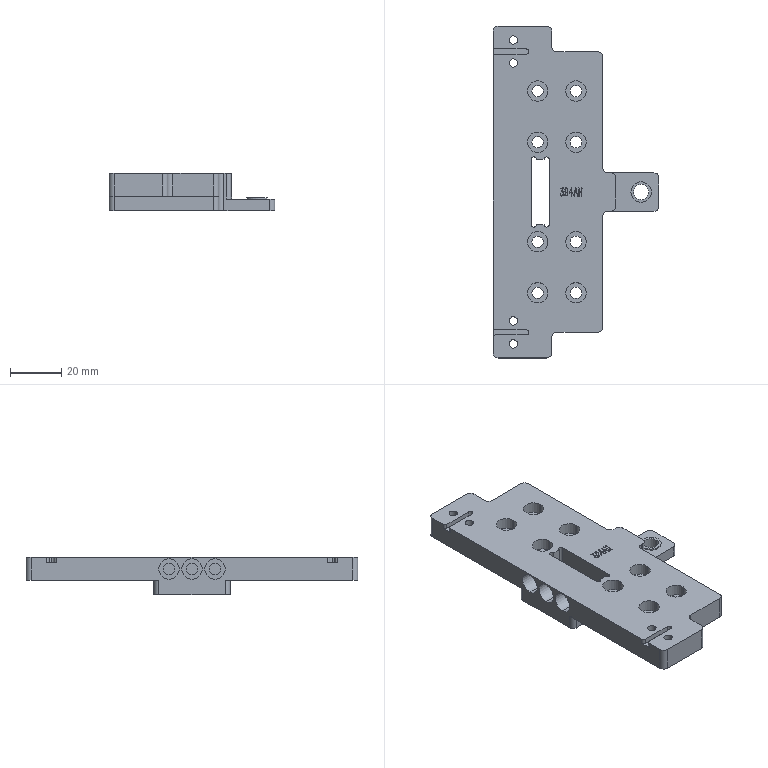Part | 1 solid | 281 faces | box 65 x 130 x 14.5 mm | volume 43349 mm3 | plane 140 | cylinder 90 | spline 51 | commonest cylinder face diameters 8 x24 4.5 x22 4 x18 2 x16 3.3 x8 6 x2